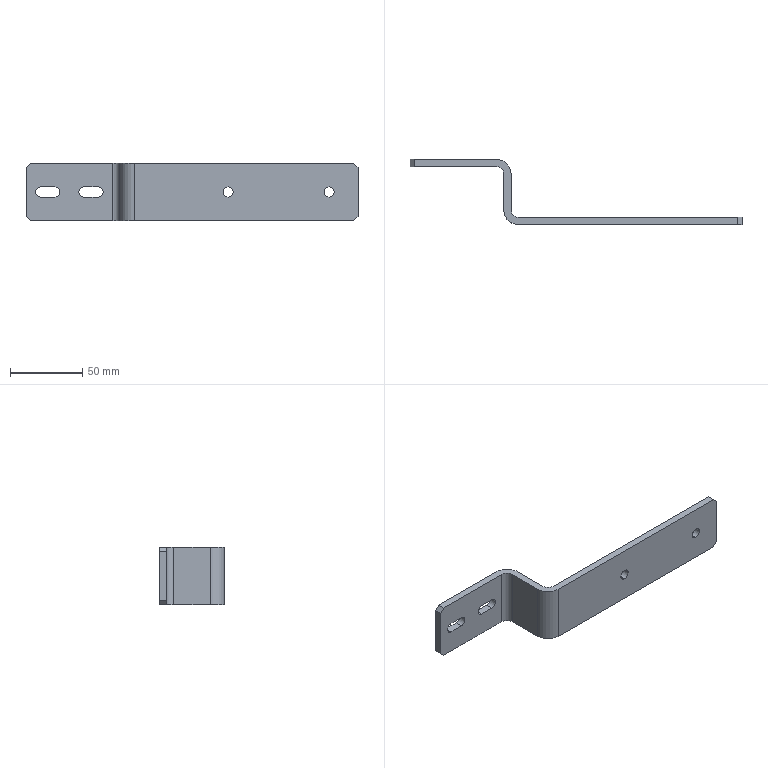Part | SolidWorks | features ICE 2, Chamfer 1, Extrusion 1 | 1 solid | 30 faces | box 230 x 45 x 40 mm | volume 51153 mm3 | plane 18 | cylinder 12 | commonest cylinder face diameters 7 x8 10 x2 20 x2
STEP:
#1=CARTESIAN_POINT('',(140.,-40.,16.5));
#2=VERTEX_POINT('',#1);
#3=CARTESIAN_POINT('',(140.,-40.,23.5));
#4=VERTEX_POINT('',#3);
#5=CARTESIAN_POINT('',(140.,-40.,20.));
#6=DIRECTION('',(0.,1.,0.));
#7=DIRECTION('',(-1.,0.,0.));
#8=AXIS2_PLACEMENT_3D('',#5,#6,#7);
#9=CIRCLE('',#8,3.5);
#10=EDGE_CURVE('',#2,#4,#9,.T.);
#11=ORIENTED_EDGE('',*,*,#10,.F.);
#12=CARTESIAN_POINT('',(140.,-35.,16.5));
#13=VERTEX_POINT('',#12);
#14=CARTESIAN_POINT('',(140.,-75.,16.5));
#15=DIRECTION('',(0.,1.,0.));
#16=VECTOR('',#15,1000.);
#17=LINE('',#14,#16);
#18=EDGE_CURVE('',#2,#13,#17,.T.);
#19=ORIENTED_EDGE('',*,*,#18,.T.);
#20=CARTESIAN_POINT('',(140.,-35.,23.5));
#21=VERTEX_POINT('',#20);
#22=CARTESIAN_POINT('',(140.,-35.,20.));
#23=DIRECTION('',(0.,1.,0.));
#24=DIRECTION('',(0.,0.,1.));
#25=AXIS2_PLACEMENT_3D('',#22,#23,#24);
#26=CIRCLE('',#25,3.5);
#27=EDGE_CURVE('',#13,#21,#26,.T.);
#28=ORIENTED_EDGE('',*,*,#27,.T.);
#29=CARTESIAN_POINT('',(140.,-75.,23.5));
#30=DIRECTION('',(0.,1.,0.));
#31=VECTOR('',#30,1000.);
#32=LINE('',#29,#31);
#33=EDGE_CURVE('',#4,#21,#32,.T.);
#34=ORIENTED_EDGE('',*,*,#33,.F.);
#35=EDGE_LOOP('',(#11,#19,#28,#34));
#36=FACE_OUTER_BOUND('',#35,.T.);
#37=CARTESIAN_POINT('',(140.,-75.,20.));
#38=DIRECTION('',(0.,1.,0.));
#39=DIRECTION('',(0.,0.,1.));
#40=AXIS2_PLACEMENT_3D('',#37,#38,#39);
#41=CYLINDRICAL_SURFACE('',#40,3.5);
#42=ADVANCED_FACE('',(#36),#41,.F.);
#43=CARTESIAN_POINT('',(210.,-40.,16.5));
#44=VERTEX_POINT('',#43);
#45=CARTESIAN_POINT('',(210.,-40.,23.5));
#46=VERTEX_POINT('',#45);
#47=CARTESIAN_POINT('',(210.,-40.,20.));
#48=DIRECTION('',(0.,1.,0.));
#49=DIRECTION('',(-1.,0.,0.));
#50=AXIS2_PLACEMENT_3D('',#47,#48,#49);
#51=CIRCLE('',#50,3.5);
#52=EDGE_CURVE('',#44,#46,#51,.T.);
#53=ORIENTED_EDGE('',*,*,#52,.F.);
#54=CARTESIAN_POINT('',(210.,-35.,16.5));
#55=VERTEX_POINT('',#54);
#56=CARTESIAN_POINT('',(210.,-75.,16.5));
#57=DIRECTION('',(0.,1.,0.));
#58=VECTOR('',#57,1000.);
#59=LINE('',#56,#58);
#60=EDGE_CURVE('',#44,#55,#59,.T.);
#61=ORIENTED_EDGE('',*,*,#60,.T.);
#62=CARTESIAN_POINT('',(210.,-35.,23.5));
#63=VERTEX_POINT('',#62);
#64=CARTESIAN_POINT('',(210.,-35.,20.));
#65=DIRECTION('',(0.,1.,0.));
#66=DIRECTION('',(0.,0.,1.));
#67=AXIS2_PLACEMENT_3D('',#64,#65,#66);
#68=CIRCLE('',#67,3.5);
#69=EDGE_CURVE('',#55,#63,#68,.T.);
#70=ORIENTED_EDGE('',*,*,#69,.T.);
#71=CARTESIAN_POINT('',(210.,-75.,23.5));
#72=DIRECTION('',(0.,1.,0.));
#73=VECTOR('',#72,1000.);
#74=LINE('',#71,#73);
#75=EDGE_CURVE('',#46,#63,#74,.T.);
#76=ORIENTED_EDGE('',*,*,#75,.F.);
#77=EDGE_LOOP('',(#53,#61,#70,#76));
#78=FACE_OUTER_BOUND('',#77,.T.);
#79=CARTESIAN_POINT('',(210.,-75.,20.));
#80=DIRECTION('',(0.,1.,0.));
#81=DIRECTION('',(0.,0.,1.));
#82=AXIS2_PLACEMENT_3D('',#79,#80,#81);
#83=CYLINDRICAL_SURFACE('',#82,3.5);
#84=ADVANCED_FACE('',(#78),#83,.F.);
#85=CARTESIAN_POINT('',(140.,-35.,20.));
#86=DIRECTION('',(0.,1.,0.));
#87=DIRECTION('',(0.,0.,1.));
#88=AXIS2_PLACEMENT_3D('',#85,#86,#87);
#89=CIRCLE('',#88,3.5);
#90=EDGE_CURVE('',#21,#13,#89,.T.);
#91=ORIENTED_EDGE('',*,*,#90,.F.);
#92=ORIENTED_EDGE('',*,*,#27,.F.);
#93=EDGE_LOOP('',(#91,#92));
#94=FACE_BOUND('',#93,.T.);
#95=CARTESIAN_POINT('',(210.,-35.,20.));
#96=DIRECTION('',(0.,1.,0.));
#97=DIRECTION('',(0.,0.,1.));
#98=AXIS2_PLACEMENT_3D('',#95,#96,#97);
#99=CIRCLE('',#98,3.5);
#100=EDGE_CURVE('',#63,#55,#99,.T.);
#101=ORIENTED_EDGE('',*,*,#100,.F.);
#102=ORIENTED_EDGE('',*,*,#69,.F.);
#103=EDGE_LOOP('',(#101,#102));
#104=FACE_BOUND('',#103,.T.);
#105=CARTESIAN_POINT('',(75.,-35.,40.));
#106=VERTEX_POINT('',#105);
#107=CARTESIAN_POINT('',(227.,-35.,40.));
#108=VERTEX_POINT('',#107);
#109=CARTESIAN_POINT('',(75.,-35.,40.));
#110=DIRECTION('',(1.,0.,0.));
#111=VECTOR('',#110,1000.);
#112=LINE('',#109,#111);
#113=EDGE_CURVE('',#106,#108,#112,.T.);
#114=ORIENTED_EDGE('',*,*,#113,.T.);
#115=CARTESIAN_POINT('',(230.,-35.,37.));
#116=VERTEX_POINT('',#115);
#117=CARTESIAN_POINT('',(151.,-35.,116.));
#118=DIRECTION('',(0.7071,0.,-0.7071));
#119=VECTOR('',#118,1000.);
#120=LINE('',#117,#119);
#121=EDGE_CURVE('',#108,#116,#120,.T.);
#122=ORIENTED_EDGE('',*,*,#121,.T.);
#123=CARTESIAN_POINT('',(230.,-35.,3.));
#124=VERTEX_POINT('',#123);
#125=CARTESIAN_POINT('',(230.,-35.,40.));
#126=DIRECTION('',(0.,0.,-1.));
#127=VECTOR('',#126,1000.);
#128=LINE('',#125,#127);
#129=EDGE_CURVE('',#116,#124,#128,.T.);
#130=ORIENTED_EDGE('',*,*,#129,.T.);
#131=CARTESIAN_POINT('',(227.,-35.,0.));
#132=VERTEX_POINT('',#131);
#133=CARTESIAN_POINT('',(171.,-35.,-56.));
#134=DIRECTION('',(-0.7071,0.,-0.7071));
#135=VECTOR('',#134,1000.);
#136=LINE('',#133,#135);
#137=EDGE_CURVE('',#124,#132,#136,.T.);
#138=ORIENTED_EDGE('',*,*,#137,.T.);
#139=CARTESIAN_POINT('',(75.,-35.,0.));
#140=VERTEX_POINT('',#139);
#141=CARTESIAN_POINT('',(75.,-35.,0.));
#142=DIRECTION('',(1.,0.,0.));
#143=VECTOR('',#142,1000.);
#144=LINE('',#141,#143);
#145=EDGE_CURVE('',#140,#132,#144,.T.);
#146=ORIENTED_EDGE('',*,*,#145,.F.);
#147=CARTESIAN_POINT('',(75.,-35.,40.));
#148=DIRECTION('',(0.,0.,-1.));
#149=VECTOR('',#148,1000.);
#150=LINE('',#147,#149);
#151=EDGE_CURVE('',#106,#140,#150,.T.);
#152=ORIENTED_EDGE('',*,*,#151,.F.);
#153=EDGE_LOOP('',(#114,#122,#130,#138,#146,#152));
#154=FACE_OUTER_BOUND('',#153,.T.);
#155=CARTESIAN_POINT('',(75.,-35.,40.));
#156=DIRECTION('',(0.,1.,0.));
#157=DIRECTION('',(0.,0.,1.));
#158=AXIS2_PLACEMENT_3D('',#155,#156,#157);
#159=PLANE('',#158);
#160=ADVANCED_FACE('',(#94,#104,#154),#159,.T.);
#161=CARTESIAN_POINT('',(70.,-30.,0.));
#162=VERTEX_POINT('',#161);
#163=CARTESIAN_POINT('',(75.,-30.,0.));
#164=DIRECTION('',(0.,0.,1.));
#165=DIRECTION('',(1.,0.,0.));
#166=AXIS2_PLACEMENT_3D('',#163,#164,#165);
#167=CIRCLE('',#166,5.);
#168=EDGE_CURVE('',#162,#140,#167,.T.);
#169=ORIENTED_EDGE('',*,*,#168,.F.);
#170=CARTESIAN_POINT('',(70.,-30.,40.));
#171=VERTEX_POINT('',#170);
#172=CARTESIAN_POINT('',(70.,-30.,40.));
#173=DIRECTION('',(0.,0.,-1.));
#174=VECTOR('',#173,1000.);
#175=LINE('',#172,#174);
#176=EDGE_CURVE('',#171,#162,#175,.T.);
#177=ORIENTED_EDGE('',*,*,#176,.F.);
#178=CARTESIAN_POINT('',(75.,-30.,40.));
#179=DIRECTION('',(0.,0.,1.));
#180=DIRECTION('',(1.,0.,0.));
#181=AXIS2_PLACEMENT_3D('',#178,#179,#180);
#182=CIRCLE('',#181,5.);
#183=EDGE_CURVE('',#171,#106,#182,.T.);
#184=ORIENTED_EDGE('',*,*,#183,.T.);
#185=ORIENTED_EDGE('',*,*,#151,.T.);
#186=EDGE_LOOP('',(#169,#177,#184,#185));
#187=FACE_OUTER_BOUND('',#186,.T.);
#188=CARTESIAN_POINT('',(75.,-30.,40.));
#189=DIRECTION('',(0.,0.,-1.));
#190=DIRECTION('',(-1.,0.,0.));
#191=AXIS2_PLACEMENT_3D('',#188,#189,#190);
#192=CYLINDRICAL_SURFACE('',#191,5.);
#193=ADVANCED_FACE('',(#187),#192,.F.);
#194=CARTESIAN_POINT('',(70.,-5.,0.));
#195=VERTEX_POINT('',#194);
#196=CARTESIAN_POINT('',(70.,-5.,0.));
#197=DIRECTION('',(0.,-1.,0.));
#198=VECTOR('',#197,1000.);
#199=LINE('',#196,#198);
#200=EDGE_CURVE('',#195,#162,#199,.T.);
#201=ORIENTED_EDGE('',*,*,#200,.F.);
#202=CARTESIAN_POINT('',(70.,-5.,40.));
#203=VERTEX_POINT('',#202);
#204=CARTESIAN_POINT('',(70.,-5.,40.));
#205=DIRECTION('',(0.,0.,-1.));
#206=VECTOR('',#205,1000.);
#207=LINE('',#204,#206);
#208=EDGE_CURVE('',#203,#195,#207,.T.);
#209=ORIENTED_EDGE('',*,*,#208,.F.);
#210=CARTESIAN_POINT('',(70.,-5.,40.));
#211=DIRECTION('',(0.,-1.,0.));
#212=VECTOR('',#211,1000.);
#213=LINE('',#210,#212);
#214=EDGE_CURVE('',#203,#171,#213,.T.);
#215=ORIENTED_EDGE('',*,*,#214,.T.);
#216=ORIENTED_EDGE('',*,*,#176,.T.);
#217=EDGE_LOOP('',(#201,#209,#215,#216));
#218=FACE_OUTER_BOUND('',#217,.T.);
#219=CARTESIAN_POINT('',(70.,-5.,40.));
#220=DIRECTION('',(1.,0.,0.));
#221=DIRECTION('',(0.,0.,-1.));
#222=AXIS2_PLACEMENT_3D('',#219,#220,#221);
#223=PLANE('',#222);
#224=ADVANCED_FACE('',(#218),#223,.T.);
#225=CARTESIAN_POINT('',(60.,5.,0.));
#226=VERTEX_POINT('',#225);
#227=CARTESIAN_POINT('',(60.,-5.,0.));
#228=DIRECTION('',(0.,0.,-1.));
#229=DIRECTION('',(-1.,0.,0.));
#230=AXIS2_PLACEMENT_3D('',#227,#228,#229);
#231=CIRCLE('',#230,10.);
#232=EDGE_CURVE('',#226,#195,#231,.T.);
#233=ORIENTED_EDGE('',*,*,#232,.F.);
#234=CARTESIAN_POINT('',(60.,5.,40.));
#235=VERTEX_POINT('',#234);
#236=CARTESIAN_POINT('',(60.,5.,40.));
#237=DIRECTION('',(0.,0.,-1.));
#238=VECTOR('',#237,1000.);
#239=LINE('',#236,#238);
#240=EDGE_CURVE('',#235,#226,#239,.T.);
#241=ORIENTED_EDGE('',*,*,#240,.F.);
#242=CARTESIAN_POINT('',(60.,-5.,40.));
#243=DIRECTION('',(0.,0.,-1.));
#244=DIRECTION('',(-1.,0.,0.));
#245=AXIS2_PLACEMENT_3D('',#242,#243,#244);
#246=CIRCLE('',#245,10.);
#247=EDGE_CURVE('',#235,#203,#246,.T.);
#248=ORIENTED_EDGE('',*,*,#247,.T.);
#249=ORIENTED_EDGE('',*,*,#208,.T.);
#250=EDGE_LOOP('',(#233,#241,#248,#249));
#251=FACE_OUTER_BOUND('',#250,.T.);
#252=CARTESIAN_POINT('',(60.,-5.,40.));
#253=DIRECTION('',(0.,0.,-1.));
#254=DIRECTION('',(-1.,0.,0.));
#255=AXIS2_PLACEMENT_3D('',#252,#253,#254);
#256=CYLINDRICAL_SURFACE('',#255,10.);
#257=ADVANCED_FACE('',(#251),#256,.T.);
#258=CARTESIAN_POINT('',(10.,5.,16.5));
#259=VERTEX_POINT('',#258);
#260=CARTESIAN_POINT('',(10.,5.,23.5));
#261=VERTEX_POINT('',#260);
#262=CARTESIAN_POINT('',(10.,5.,20.));
#263=DIRECTION('',(0.,1.,0.));
#264=DIRECTION('',(0.,0.,1.));
#265=AXIS2_PLACEMENT_3D('',#262,#263,#264);
#266=CIRCLE('',#265,3.5);
#267=EDGE_CURVE('',#259,#261,#266,.T.);
#268=ORIENTED_EDGE('',*,*,#267,.F.);
#269=CARTESIAN_POINT('',(20.,5.,16.5));
#270=VERTEX_POINT('',#269);
#271=CARTESIAN_POINT('',(10.,5.,16.5));
#272=DIRECTION('',(-1.,0.,0.));
#273=VECTOR('',#272,1000.);
#274=LINE('',#271,#273);
#275=EDGE_CURVE('',#270,#259,#274,.T.);
#276=ORIENTED_EDGE('',*,*,#275,.F.);
#277=CARTESIAN_POINT('',(20.,5.,23.5));
#278=VERTEX_POINT('',#277);
#279=CARTESIAN_POINT('',(20.,5.,20.));
#280=DIRECTION('',(0.,1.,0.));
#281=DIRECTION('',(0.,0.,1.));
#282=AXIS2_PLACEMENT_3D('',#279,#280,#281);
#283=CIRCLE('',#282,3.5);
#284=EDGE_CURVE('',#278,#270,#283,.T.);
#285=ORIENTED_EDGE('',*,*,#284,.F.);
#286=CARTESIAN_POINT('',(10.,5.,23.5));
#287=DIRECTION('',(1.,0.,0.));
#288=VECTOR('',#287,1000.);
#289=LINE('',#286,#288);
#290=EDGE_CURVE('',#261,#278,#289,.T.);
#291=ORIENTED_EDGE('',*,*,#290,.F.);
#292=EDGE_LOOP('',(#268,#276,#285,#291));
#293=FACE_BOUND('',#292,.T.);
#294=CARTESIAN_POINT('',(40.,5.,16.5));
#295=VERTEX_POINT('',#294);
#296=CARTESIAN_POINT('',(40.,5.,23.5));
#297=VERTEX_POINT('',#296);
#298=CARTESIAN_POINT('',(40.,5.,20.));
#299=DIRECTION('',(0.,1.,0.));
#300=DIRECTION('',(0.,0.,1.));
#301=AXIS2_PLACEMENT_3D('',#298,#299,#300);
#302=CIRCLE('',#301,3.5);
#303=EDGE_CURVE('',#295,#297,#302,.T.);
#304=ORIENTED_EDGE('',*,*,#303,.F.);
#305=CARTESIAN_POINT('',(50.,5.,16.5));
#306=VERTEX_POINT('',#305);
#307=CARTESIAN_POINT('',(40.,5.,16.5));
#308=DIRECTION('',(-1.,0.,0.));
#309=VECTOR('',#308,1000.);
#310=LINE('',#307,#309);
#311=EDGE_CURVE('',#306,#295,#310,.T.);
#312=ORIENTED_EDGE('',*,*,#311,.F.);
#313=CARTESIAN_POINT('',(50.,5.,23.5));
#314=VERTEX_POINT('',#313);
#315=CARTESIAN_POINT('',(50.,5.,20.));
#316=DIRECTION('',(0.,1.,0.));
#317=DIRECTION('',(0.,0.,1.));
#318=AXIS2_PLACEMENT_3D('',#315,#316,#317);
#319=CIRCLE('',#318,3.5);
#320=EDGE_CURVE('',#314,#306,#319,.T.);
#321=ORIENTED_EDGE('',*,*,#320,.F.);
#322=CARTESIAN_POINT('',(40.,5.,23.5));
#323=DIRECTION('',(1.,0.,0.));
#324=VECTOR('',#323,1000.);
#325=LINE('',#322,#324);
#326=EDGE_CURVE('',#297,#314,#325,.T.);
#327=ORIENTED_EDGE('',*,*,#326,.F.);
#328=EDGE_LOOP('',(#304,#312,#321,#327));
#329=FACE_BOUND('',#328,.T.);
#330=CARTESIAN_POINT('',(0.,5.,37.));
#331=VERTEX_POINT('',#330);
#332=CARTESIAN_POINT('',(0.,5.,3.));
#333=VERTEX_POINT('',#332);
#334=CARTESIAN_POINT('',(0.,5.,40.));
#335=DIRECTION('',(0.,0.,-1.));
#336=VECTOR('',#335,1000.);
#337=LINE('',#334,#336);
#338=EDGE_CURVE('',#331,#333,#337,.T.);
#339=ORIENTED_EDGE('',*,*,#338,.F.);
#340=CARTESIAN_POINT('',(3.,5.,40.));
#341=VERTEX_POINT('',#340);
#342=CARTESIAN_POINT('',(1.5,5.,38.5));
#343=DIRECTION('',(0.7071,0.,0.7071));
#344=VECTOR('',#343,1000.);
#345=LINE('',#342,#344);
#346=EDGE_CURVE('',#331,#341,#345,.T.);
#347=ORIENTED_EDGE('',*,*,#346,.T.);
#348=CARTESIAN_POINT('',(0.,5.,40.));
#349=DIRECTION('',(1.,0.,0.));
#350=VECTOR('',#349,1000.);
#351=LINE('',#348,#350);
#352=EDGE_CURVE('',#341,#235,#351,.T.);
#353=ORIENTED_EDGE('',*,*,#352,.T.);
#354=ORIENTED_EDGE('',*,*,#240,.T.);
#355=CARTESIAN_POINT('',(3.,5.,0.));
#356=VERTEX_POINT('',#355);
#357=CARTESIAN_POINT('',(0.,5.,0.));
#358=DIRECTION('',(1.,0.,0.));
#359=VECTOR('',#358,1000.);
#360=LINE('',#357,#359);
#361=EDGE_CURVE('',#356,#226,#360,.T.);
#362=ORIENTED_EDGE('',*,*,#361,.F.);
#363=CARTESIAN_POINT('',(-18.5,5.,21.5));
#364=DIRECTION('',(-0.7071,0.,0.7071));
#365=VECTOR('',#364,1000.);
#366=LINE('',#363,#365);
#367=EDGE_CURVE('',#356,#333,#366,.T.);
#368=ORIENTED_EDGE('',*,*,#367,.T.);
#369=EDGE_LOOP('',(#339,#347,#353,#354,#362,#368));
#370=FACE_OUTER_BOUND('',#369,.T.);
#371=CARTESIAN_POINT('',(0.,5.,40.));
#372=DIRECTION('',(0.,1.,0.));
#373=DIRECTION('',(0.,0.,1.));
#374=AXIS2_PLACEMENT_3D('',#371,#372,#373);
#375=PLANE('',#374);
#376=ADVANCED_FACE('',(#293,#329,#370),#375,.T.);
#377=CARTESIAN_POINT('',(0.,0.,37.));
#378=VERTEX_POINT('',#377);
#379=CARTESIAN_POINT('',(0.,0.,3.));
#380=VERTEX_POINT('',#379);
#381=CARTESIAN_POINT('',(0.,0.,40.));
#382=DIRECTION('',(0.,0.,-1.));
#383=VECTOR('',#382,1000.);
#384=LINE('',#381,#383);
#385=EDGE_CURVE('',#378,#380,#384,.T.);
#386=ORIENTED_EDGE('',*,*,#385,.F.);
#387=CARTESIAN_POINT('',(0.,5.,37.));
#388=DIRECTION('',(0.,1.,0.));
#389=VECTOR('',#388,1000.);
#390=LINE('',#387,#389);
#391=EDGE_CURVE('',#378,#331,#390,.T.);
#392=ORIENTED_EDGE('',*,*,#391,.T.);
#393=ORIENTED_EDGE('',*,*,#338,.T.);
#394=CARTESIAN_POINT('',(0.,5.,3.));
#395=DIRECTION('',(0.,-1.,0.));
#396=VECTOR('',#395,1000.);
#397=LINE('',#394,#396);
#398=EDGE_CURVE('',#333,#380,#397,.T.);
#399=ORIENTED_EDGE('',*,*,#398,.T.);
#400=EDGE_LOOP('',(#386,#392,#393,#399));
#401=FACE_OUTER_BOUND('',#400,.T.);
#402=CARTESIAN_POINT('',(0.,5.,40.));
#403=DIRECTION('',(1.,0.,0.));
#404=DIRECTION('',(0.,0.,-1.));
#405=AXIS2_PLACEMENT_3D('',#402,#403,#404);
#406=PLANE('',#405);
#407=ADVANCED_FACE('',(#401),#406,.F.);
#408=CARTESIAN_POINT('',(20.,0.,16.5));
#409=VERTEX_POINT('',#408);
#410=CARTESIAN_POINT('',(10.,0.,16.5));
#411=VERTEX_POINT('',#410);
#412=CARTESIAN_POINT('',(0.,0.,16.5));
#413=DIRECTION('',(-1.,0.,0.));
#414=VECTOR('',#413,1000.);
#415=LINE('',#412,#414);
#416=EDGE_CURVE('',#409,#411,#415,.T.);
#417=ORIENTED_EDGE('',*,*,#416,.T.);
#418=CARTESIAN_POINT('',(10.,0.,23.5));
#419=VERTEX_POINT('',#418);
#420=CARTESIAN_POINT('',(10.,0.,20.));
#421=DIRECTION('',(0.,1.,0.));
#422=DIRECTION('',(0.,0.,1.));
#423=AXIS2_PLACEMENT_3D('',#420,#421,#422);
#424=CIRCLE('',#423,3.5);
#425=EDGE_CURVE('',#411,#419,#424,.T.);
#426=ORIENTED_EDGE('',*,*,#425,.T.);
#427=CARTESIAN_POINT('',(20.,0.,23.5));
#428=VERTEX_POINT('',#427);
#429=CARTESIAN_POINT('',(0.,0.,23.5));
#430=DIRECTION('',(1.,0.,0.));
#431=VECTOR('',#430,1000.);
#432=LINE('',#429,#431);
#433=EDGE_CURVE('',#419,#428,#432,.T.);
#434=ORIENTED_EDGE('',*,*,#433,.T.);
#435=CARTESIAN_POINT('',(20.,0.,20.));
#436=DIRECTION('',(0.,1.,0.));
#437=DIRECTION('',(0.,0.,1.));
#438=AXIS2_PLACEMENT_3D('',#435,#436,#437);
#439=CIRCLE('',#438,3.5);
#440=EDGE_CURVE('',#428,#409,#439,.T.);
#441=ORIENTED_EDGE('',*,*,#440,.T.);
#442=EDGE_LOOP('',(#417,#426,#434,#441));
#443=FACE_BOUND('',#442,.T.);
#444=CARTESIAN_POINT('',(50.,0.,16.5));
#445=VERTEX_POINT('',#444);
#446=CARTESIAN_POINT('',(40.,0.,16.5));
#447=VERTEX_POINT('',#446);
#448=CARTESIAN_POINT('',(0.,0.,16.5));
#449=DIRECTION('',(-1.,0.,0.));
#450=VECTOR('',#449,1000.);
#451=LINE('',#448,#450);
#452=EDGE_CURVE('',#445,#447,#451,.T.);
#453=ORIENTED_EDGE('',*,*,#452,.T.);
#454=CARTESIAN_POINT('',(40.,0.,23.5));
#455=VERTEX_POINT('',#454);
#456=CARTESIAN_POINT('',(40.,0.,20.));
#457=DIRECTION('',(0.,1.,0.));
#458=DIRECTION('',(0.,0.,1.));
#459=AXIS2_PLACEMENT_3D('',#456,#457,#458);
#460=CIRCLE('',#459,3.5);
#461=EDGE_CURVE('',#447,#455,#460,.T.);
#462=ORIENTED_EDGE('',*,*,#461,.T.);
#463=CARTESIAN_POINT('',(50.,0.,23.5));
#464=VERTEX_POINT('',#463);
#465=CARTESIAN_POINT('',(0.,0.,23.5));
#466=DIRECTION('',(1.,0.,0.));
#467=VECTOR('',#466,1000.);
#468=LINE('',#465,#467);
#469=EDGE_CURVE('',#455,#464,#468,.T.);
#470=ORIENTED_EDGE('',*,*,#469,.T.);
#471=CARTESIAN_POINT('',(50.,0.,20.));
#472=DIRECTION('',(0.,1.,0.));
#473=DIRECTION('',(0.,0.,1.));
#474=AXIS2_PLACEMENT_3D('',#471,#472,#473);
#475=CIRCLE('',#474,3.5);
#476=EDGE_CURVE('',#464,#445,#475,.T.);
#477=ORIENTED_EDGE('',*,*,#476,.T.);
#478=EDGE_LOOP('',(#453,#462,#470,#477));
#479=FACE_BOUND('',#478,.T.);
#480=CARTESIAN_POINT('',(3.,0.,40.));
#481=VERTEX_POINT('',#480);
#482=CARTESIAN_POINT('',(60.,0.,40.));
#483=VERTEX_POINT('',#482);
#484=CARTESIAN_POINT('',(0.,0.,40.));
#485=DIRECTION('',(1.,0.,0.));
#486=VECTOR('',#485,1000.);
#487=LINE('',#484,#486);
#488=EDGE_CURVE('',#481,#483,#487,.T.);
#489=ORIENTED_EDGE('',*,*,#488,.F.);
#490=CARTESIAN_POINT('',(3.,0.,40.));
#491=DIRECTION('',(-0.7071,0.,-0.7071));
#492=VECTOR('',#491,1000.);
#493=LINE('',#490,#492);
#494=EDGE_CURVE('',#481,#378,#493,.T.);
#495=ORIENTED_EDGE('',*,*,#494,.T.);
#496=ORIENTED_EDGE('',*,*,#385,.T.);
#497=CARTESIAN_POINT('',(3.,0.,0.));
#498=VERTEX_POINT('',#497);
#499=CARTESIAN_POINT('',(0.,0.,3.));
#500=DIRECTION('',(0.7071,0.,-0.7071));
#501=VECTOR('',#500,1000.);
#502=LINE('',#499,#501);
#503=EDGE_CURVE('',#380,#498,#502,.T.);
#504=ORIENTED_EDGE('',*,*,#503,.T.);
#505=CARTESIAN_POINT('',(60.,0.,0.));
#506=VERTEX_POINT('',#505);
#507=CARTESIAN_POINT('',(0.,0.,0.));
#508=DIRECTION('',(1.,0.,0.));
#509=VECTOR('',#508,1000.);
#510=LINE('',#507,#509);
#511=EDGE_CURVE('',#498,#506,#510,.T.);
#512=ORIENTED_EDGE('',*,*,#511,.T.);
#513=CARTESIAN_POINT('',(60.,0.,40.));
#514=DIRECTION('',(0.,0.,-1.));
#515=VECTOR('',#514,1000.);
#516=LINE('',#513,#515);
#517=EDGE_CURVE('',#483,#506,#516,.T.);
#518=ORIENTED_EDGE('',*,*,#517,.F.);
#519=EDGE_LOOP('',(#489,#495,#496,#504,#512,#518));
#520=FACE_OUTER_BOUND('',#519,.T.);
#521=CARTESIAN_POINT('',(0.,0.,40.));
#522=DIRECTION('',(0.,1.,0.));
#523=DIRECTION('',(0.,0.,1.));
#524=AXIS2_PLACEMENT_3D('',#521,#522,#523);
#525=PLANE('',#524);
#526=ADVANCED_FACE('',(#443,#479,#520),#525,.F.);
#527=CARTESIAN_POINT('',(65.,-5.,0.));
#528=VERTEX_POINT('',#527);
#529=CARTESIAN_POINT('',(60.,-5.,0.));
#530=DIRECTION('',(0.,0.,-1.));
#531=DIRECTION('',(-1.,0.,0.));
#532=AXIS2_PLACEMENT_3D('',#529,#530,#531);
#533=CIRCLE('',#532,5.);
#534=EDGE_CURVE('',#506,#528,#533,.T.);
#535=ORIENTED_EDGE('',*,*,#534,.T.);
#536=CARTESIAN_POINT('',(65.,-5.,40.));
#537=VERTEX_POINT('',#536);
#538=CARTESIAN_POINT('',(65.,-5.,40.));
#539=DIRECTION('',(0.,0.,-1.));
#540=VECTOR('',#539,1000.);
#541=LINE('',#538,#540);
#542=EDGE_CURVE('',#537,#528,#541,.T.);
#543=ORIENTED_EDGE('',*,*,#542,.F.);
#544=CARTESIAN_POINT('',(60.,-5.,40.));
#545=DIRECTION('',(0.,0.,-1.));
#546=DIRECTION('',(-1.,0.,0.));
#547=AXIS2_PLACEMENT_3D('',#544,#545,#546);
#548=CIRCLE('',#547,5.);
#549=EDGE_CURVE('',#483,#537,#548,.T.);
#550=ORIENTED_EDGE('',*,*,#549,.F.);
#551=ORIENTED_EDGE('',*,*,#517,.T.);
#552=EDGE_LOOP('',(#535,#543,#550,#551));
#553=FACE_OUTER_BOUND('',#552,.T.);
#554=CARTESIAN_POINT('',(60.,-5.,40.));
#555=DIRECTION('',(0.,0.,-1.));
#556=DIRECTION('',(-1.,0.,0.));
#557=AXIS2_PLACEMENT_3D('',#554,#555,#556);
#558=CYLINDRICAL_SURFACE('',#557,5.);
#559=ADVANCED_FACE('',(#553),#558,.F.);
#560=CARTESIAN_POINT('',(65.,-30.,0.));
#561=VERTEX_POINT('',#560);
#562=CARTESIAN_POINT('',(65.,-5.,0.));
#563=DIRECTION('',(0.,-1.,0.));
#564=VECTOR('',#563,1000.);
#565=LINE('',#562,#564);
#566=EDGE_CURVE('',#528,#561,#565,.T.);
#567=ORIENTED_EDGE('',*,*,#566,.T.);
#568=CARTESIAN_POINT('',(65.,-30.,40.));
#569=VERTEX_POINT('',#568);
#570=CARTESIAN_POINT('',(65.,-30.,40.));
#571=DIRECTION('',(0.,0.,-1.));
#572=VECTOR('',#571,1000.);
#573=LINE('',#570,#572);
#574=EDGE_CURVE('',#569,#561,#573,.T.);
#575=ORIENTED_EDGE('',*,*,#574,.F.);
#576=CARTESIAN_POINT('',(65.,-5.,40.));
#577=DIRECTION('',(0.,-1.,0.));
#578=VECTOR('',#577,1000.);
#579=LINE('',#576,#578);
#580=EDGE_CURVE('',#537,#569,#579,.T.);
#581=ORIENTED_EDGE('',*,*,#580,.F.);
#582=ORIENTED_EDGE('',*,*,#542,.T.);
#583=EDGE_LOOP('',(#567,#575,#581,#582));
#584=FACE_OUTER_BOUND('',#583,.T.);
#585=CARTESIAN_POINT('',(65.,-5.,40.));
#586=DIRECTION('',(1.,0.,0.));
#587=DIRECTION('',(0.,1.,0.));
#588=AXIS2_PLACEMENT_3D('',#585,#586,#587);
#589=PLANE('',#588);
#590=ADVANCED_FACE('',(#584),#589,.F.);
#591=CARTESIAN_POINT('',(75.,-40.,0.));
#592=VERTEX_POINT('',#591);
#593=CARTESIAN_POINT('',(75.,-30.,0.));
#594=DIRECTION('',(0.,0.,1.));
#595=DIRECTION('',(1.,0.,0.));
#596=AXIS2_PLACEMENT_3D('',#593,#594,#595);
#597=CIRCLE('',#596,10.);
#598=EDGE_CURVE('',#561,#592,#597,.T.);
#599=ORIENTED_EDGE('',*,*,#598,.T.);
#600=CARTESIAN_POINT('',(75.,-40.,40.));
#601=VERTEX_POINT('',#600);
#602=CARTESIAN_POINT('',(75.,-40.,40.));
#603=DIRECTION('',(0.,0.,-1.));
#604=VECTOR('',#603,1000.);
#605=LINE('',#602,#604);
#606=EDGE_CURVE('',#601,#592,#605,.T.);
#607=ORIENTED_EDGE('',*,*,#606,.F.);
#608=CARTESIAN_POINT('',(75.,-30.,40.));
#609=DIRECTION('',(0.,0.,1.));
#610=DIRECTION('',(1.,0.,0.));
#611=AXIS2_PLACEMENT_3D('',#608,#609,#610);
#612=CIRCLE('',#611,10.);
#613=EDGE_CURVE('',#569,#601,#612,.T.);
#614=ORIENTED_EDGE('',*,*,#613,.F.);
#615=ORIENTED_EDGE('',*,*,#574,.T.);
#616=EDGE_LOOP('',(#599,#607,#614,#615));
#617=FACE_OUTER_BOUND('',#616,.T.);
#618=CARTESIAN_POINT('',(75.,-30.,40.));
#619=DIRECTION('',(0.,0.,-1.));
#620=DIRECTION('',(-1.,0.,0.));
#621=AXIS2_PLACEMENT_3D('',#618,#619,#620);
#622=CYLINDRICAL_SURFACE('',#621,10.);
#623=ADVANCED_FACE('',(#617),#622,.T.);
#624=CARTESIAN_POINT('',(140.,-40.,20.));
#625=DIRECTION('',(0.,1.,0.));
#626=DIRECTION('',(-1.,0.,0.));
#627=AXIS2_PLACEMENT_3D('',#624,#625,#626);
#628=CIRCLE('',#627,3.5);
#629=EDGE_CURVE('',#4,#2,#628,.T.);
#630=ORIENTED_EDGE('',*,*,#629,.T.);
#631=ORIENTED_EDGE('',*,*,#10,.T.);
#632=EDGE_LOOP('',(#630,#631));
#633=FACE_BOUND('',#632,.T.);
#634=CARTESIAN_POINT('',(210.,-40.,20.));
#635=DIRECTION('',(0.,1.,0.));
#636=DIRECTION('',(-1.,0.,0.));
#637=AXIS2_PLACEMENT_3D('',#634,#635,#636);
#638=CIRCLE('',#637,3.5);
#639=EDGE_CURVE('',#46,#44,#638,.T.);
#640=ORIENTED_EDGE('',*,*,#639,.T.);
#641=ORIENTED_EDGE('',*,*,#52,.T.);
#642=EDGE_LOOP('',(#640,#641));
#643=FACE_BOUND('',#642,.T.);
#644=CARTESIAN_POINT('',(230.,-40.,37.));
#645=VERTEX_POINT('',#644);
#646=CARTESIAN_POINT('',(230.,-40.,3.));
#647=VERTEX_POINT('',#646);
#648=CARTESIAN_POINT('',(230.,-40.,40.));
#649=DIRECTION('',(0.,0.,-1.));
#650=VECTOR('',#649,1000.);
#651=LINE('',#648,#650);
#652=EDGE_CURVE('',#645,#647,#651,.T.);
#653=ORIENTED_EDGE('',*,*,#652,.F.);
#654=CARTESIAN_POINT('',(227.,-40.,40.));
#655=VERTEX_POINT('',#654);
#656=CARTESIAN_POINT('',(230.,-40.,37.));
#657=DIRECTION('',(-0.7071,0.,0.7071));
#658=VECTOR('',#657,1000.);
#659=LINE('',#656,#658);
#660=EDGE_CURVE('',#645,#655,#659,.T.);
#661=ORIENTED_EDGE('',*,*,#660,.T.);
#662=CARTESIAN_POINT('',(75.,-40.,40.));
#663=DIRECTION('',(1.,0.,0.));
#664=VECTOR('',#663,1000.);
#665=LINE('',#662,#664);
#666=EDGE_CURVE('',#601,#655,#665,.T.);
#667=ORIENTED_EDGE('',*,*,#666,.F.);
#668=ORIENTED_EDGE('',*,*,#606,.T.);
#669=CARTESIAN_POINT('',(227.,-40.,0.));
#670=VERTEX_POINT('',#669);
#671=CARTESIAN_POINT('',(75.,-40.,0.));
#672=DIRECTION('',(1.,0.,0.));
#673=VECTOR('',#672,1000.);
#674=LINE('',#671,#673);
#675=EDGE_CURVE('',#592,#670,#674,.T.);
#676=ORIENTED_EDGE('',*,*,#675,.T.);
#677=CARTESIAN_POINT('',(227.,-40.,0.));
#678=DIRECTION('',(0.7071,0.,0.7071));
#679=VECTOR('',#678,1000.);
#680=LINE('',#677,#679);
#681=EDGE_CURVE('',#670,#647,#680,.T.);
#682=ORIENTED_EDGE('',*,*,#681,.T.);
#683=EDGE_LOOP('',(#653,#661,#667,#668,#676,#682));
#684=FACE_OUTER_BOUND('',#683,.T.);
#685=CARTESIAN_POINT('',(75.,-40.,40.));
#686=DIRECTION('',(0.,1.,0.));
#687=DIRECTION('',(-1.,0.,0.));
#688=AXIS2_PLACEMENT_3D('',#685,#686,#687);
#689=PLANE('',#688);
#690=ADVANCED_FACE('',(#633,#643,#684),#689,.F.);
#691=ORIENTED_EDGE('',*,*,#129,.F.);
#692=CARTESIAN_POINT('',(230.,-35.,37.));
#693=DIRECTION('',(0.,-1.,0.));
#694=VECTOR('',#693,1000.);
#695=LINE('',#692,#694);
#696=EDGE_CURVE('',#116,#645,#695,.T.);
#697=ORIENTED_EDGE('',*,*,#696,.T.);
#698=ORIENTED_EDGE('',*,*,#652,.T.);
#699=CARTESIAN_POINT('',(230.,-35.,3.));
#700=DIRECTION('',(0.,1.,0.));
#701=VECTOR('',#700,1000.);
#702=LINE('',#699,#701);
#703=EDGE_CURVE('',#647,#124,#702,.T.);
#704=ORIENTED_EDGE('',*,*,#703,.T.);
#705=EDGE_LOOP('',(#691,#697,#698,#704));
#706=FACE_OUTER_BOUND('',#705,.T.);
#707=CARTESIAN_POINT('',(230.,-35.,40.));
#708=DIRECTION('',(1.,0.,0.));
#709=DIRECTION('',(0.,0.,-1.));
#710=AXIS2_PLACEMENT_3D('',#707,#708,#709);
#711=PLANE('',#710);
#712=ADVANCED_FACE('',(#706),#711,.T.);
#713=ORIENTED_EDGE('',*,*,#352,.F.);
#714=CARTESIAN_POINT('',(3.,0.,40.));
#715=DIRECTION('',(0.,-1.,0.));
#716=VECTOR('',#715,1000.);
#717=LINE('',#714,#716);
#718=EDGE_CURVE('',#341,#481,#717,.T.);
#719=ORIENTED_EDGE('',*,*,#718,.T.);
#720=ORIENTED_EDGE('',*,*,#488,.T.);
#721=ORIENTED_EDGE('',*,*,#549,.T.);
#722=ORIENTED_EDGE('',*,*,#580,.T.);
#723=ORIENTED_EDGE('',*,*,#613,.T.);
#724=ORIENTED_EDGE('',*,*,#666,.T.);
#725=CARTESIAN_POINT('',(227.,-30.,40.));
#726=DIRECTION('',(0.,1.,0.));
#727=VECTOR('',#726,1000.);
#728=LINE('',#725,#727);
#729=EDGE_CURVE('',#655,#108,#728,.T.);
#730=ORIENTED_EDGE('',*,*,#729,.T.);
#731=ORIENTED_EDGE('',*,*,#113,.F.);
#732=ORIENTED_EDGE('',*,*,#183,.F.);
#733=ORIENTED_EDGE('',*,*,#214,.F.);
#734=ORIENTED_EDGE('',*,*,#247,.F.);
#735=EDGE_LOOP('',(#713,#719,#720,#721,#722,#723,#724,#730,#731,#732,#733,#734));
#736=FACE_OUTER_BOUND('',#735,.T.);
#737=CARTESIAN_POINT('',(75.,-30.,40.));
#738=DIRECTION('',(0.,0.,1.));
#739=DIRECTION('',(1.,0.,0.));
#740=AXIS2_PLACEMENT_3D('',#737,#738,#739);
#741=PLANE('',#740);
#742=ADVANCED_FACE('',(#736),#741,.T.);
#743=ORIENTED_EDGE('',*,*,#511,.F.);
#744=CARTESIAN_POINT('',(3.,-30.,0.));
#745=DIRECTION('',(0.,1.,0.));
#746=VECTOR('',#745,1000.);
#747=LINE('',#744,#746);
#748=EDGE_CURVE('',#498,#356,#747,.T.);
#749=ORIENTED_EDGE('',*,*,#748,.T.);
#750=ORIENTED_EDGE('',*,*,#361,.T.);
#751=ORIENTED_EDGE('',*,*,#232,.T.);
#752=ORIENTED_EDGE('',*,*,#200,.T.);
#753=ORIENTED_EDGE('',*,*,#168,.T.);
#754=ORIENTED_EDGE('',*,*,#145,.T.);
#755=CARTESIAN_POINT('',(227.,-40.,0.));
#756=DIRECTION('',(0.,-1.,0.));
#757=VECTOR('',#756,1000.);
#758=LINE('',#755,#757);
#759=EDGE_CURVE('',#132,#670,#758,.T.);
#760=ORIENTED_EDGE('',*,*,#759,.T.);
#761=ORIENTED_EDGE('',*,*,#675,.F.);
#762=ORIENTED_EDGE('',*,*,#598,.F.);
#763=ORIENTED_EDGE('',*,*,#566,.F.);
#764=ORIENTED_EDGE('',*,*,#534,.F.);
#765=EDGE_LOOP('',(#743,#749,#750,#751,#752,#753,#754,#760,#761,#762,#763,#764));
#766=FACE_OUTER_BOUND('',#765,.T.);
#767=CARTESIAN_POINT('',(75.,-30.,0.));
#768=DIRECTION('',(0.,0.,1.));
#769=DIRECTION('',(1.,0.,0.));
#770=AXIS2_PLACEMENT_3D('',#767,#768,#769);
#771=PLANE('',#770);
#772=ADVANCED_FACE('',(#766),#771,.F.);
#773=CARTESIAN_POINT('',(40.,-35.,16.5));
#774=DIRECTION('',(0.,1.,0.));
#775=VECTOR('',#774,1000.);
#776=LINE('',#773,#775);
#777=EDGE_CURVE('',#447,#295,#776,.T.);
#778=ORIENTED_EDGE('',*,*,#777,.T.);
#779=ORIENTED_EDGE('',*,*,#303,.T.);
#780=CARTESIAN_POINT('',(40.,-35.,23.5));
#781=DIRECTION('',(0.,1.,0.));
#782=VECTOR('',#781,1000.);
#783=LINE('',#780,#782);
#784=EDGE_CURVE('',#455,#297,#783,.T.);
#785=ORIENTED_EDGE('',*,*,#784,.F.);
#786=ORIENTED_EDGE('',*,*,#461,.F.);
#787=EDGE_LOOP('',(#778,#779,#785,#786));
#788=FACE_OUTER_BOUND('',#787,.T.);
#789=CARTESIAN_POINT('',(40.,-35.,20.));
#790=DIRECTION('',(0.,1.,0.));
#791=DIRECTION('',(0.,0.,1.));
#792=AXIS2_PLACEMENT_3D('',#789,#790,#791);
#793=CYLINDRICAL_SURFACE('',#792,3.5);
#794=ADVANCED_FACE('',(#788),#793,.F.);
#795=CARTESIAN_POINT('',(50.,-35.,16.5));
#796=DIRECTION('',(0.,1.,0.));
#797=VECTOR('',#796,1000.);
#798=LINE('',#795,#797);
#799=EDGE_CURVE('',#445,#306,#798,.T.);
#800=ORIENTED_EDGE('',*,*,#799,.T.);
#801=ORIENTED_EDGE('',*,*,#311,.T.);
#802=ORIENTED_EDGE('',*,*,#777,.F.);
#803=ORIENTED_EDGE('',*,*,#452,.F.);
#804=EDGE_LOOP('',(#800,#801,#802,#803));
#805=FACE_OUTER_BOUND('',#804,.T.);
#806=CARTESIAN_POINT('',(40.,-35.,16.5));
#807=DIRECTION('',(0.,0.,-1.));
#808=DIRECTION('',(-1.,0.,0.));
#809=AXIS2_PLACEMENT_3D('',#806,#807,#808);
#810=PLANE('',#809);
#811=ADVANCED_FACE('',(#805),#810,.F.);
#812=CARTESIAN_POINT('',(50.,-35.,23.5));
#813=DIRECTION('',(0.,1.,0.));
#814=VECTOR('',#813,1000.);
#815=LINE('',#812,#814);
#816=EDGE_CURVE('',#464,#314,#815,.T.);
#817=ORIENTED_EDGE('',*,*,#816,.T.);
#818=ORIENTED_EDGE('',*,*,#320,.T.);
#819=ORIENTED_EDGE('',*,*,#799,.F.);
#820=ORIENTED_EDGE('',*,*,#476,.F.);
#821=EDGE_LOOP('',(#817,#818,#819,#820));
#822=FACE_OUTER_BOUND('',#821,.T.);
#823=CARTESIAN_POINT('',(50.,-35.,20.));
#824=DIRECTION('',(0.,1.,0.));
#825=DIRECTION('',(0.,0.,1.));
#826=AXIS2_PLACEMENT_3D('',#823,#824,#825);
#827=CYLINDRICAL_SURFACE('',#826,3.5);
#828=ADVANCED_FACE('',(#822),#827,.F.);
#829=ORIENTED_EDGE('',*,*,#784,.T.);
#830=ORIENTED_EDGE('',*,*,#326,.T.);
#831=ORIENTED_EDGE('',*,*,#816,.F.);
#832=ORIENTED_EDGE('',*,*,#469,.F.);
#833=EDGE_LOOP('',(#829,#830,#831,#832));
#834=FACE_OUTER_BOUND('',#833,.T.);
#835=CARTESIAN_POINT('',(40.,-35.,23.5));
#836=DIRECTION('',(0.,0.,1.));
#837=DIRECTION('',(1.,0.,0.));
#838=AXIS2_PLACEMENT_3D('',#835,#836,#837);
#839=PLANE('',#838);
#840=ADVANCED_FACE('',(#834),#839,.F.);
#841=CARTESIAN_POINT('',(10.,-35.,16.5));
#842=DIRECTION('',(0.,1.,0.));
#843=VECTOR('',#842,1000.);
#844=LINE('',#841,#843);
#845=EDGE_CURVE('',#411,#259,#844,.T.);
#846=ORIENTED_EDGE('',*,*,#845,.T.);
#847=ORIENTED_EDGE('',*,*,#267,.T.);
#848=CARTESIAN_POINT('',(10.,-35.,23.5));
#849=DIRECTION('',(0.,1.,0.));
#850=VECTOR('',#849,1000.);
#851=LINE('',#848,#850);
#852=EDGE_CURVE('',#419,#261,#851,.T.);
#853=ORIENTED_EDGE('',*,*,#852,.F.);
#854=ORIENTED_EDGE('',*,*,#425,.F.);
#855=EDGE_LOOP('',(#846,#847,#853,#854));
#856=FACE_OUTER_BOUND('',#855,.T.);
#857=CARTESIAN_POINT('',(10.,-35.,20.));
#858=DIRECTION('',(0.,1.,0.));
#859=DIRECTION('',(0.,0.,1.));
#860=AXIS2_PLACEMENT_3D('',#857,#858,#859);
#861=CYLINDRICAL_SURFACE('',#860,3.5);
#862=ADVANCED_FACE('',(#856),#861,.F.);
#863=CARTESIAN_POINT('',(20.,-35.,16.5));
#864=DIRECTION('',(0.,1.,0.));
#865=VECTOR('',#864,1000.);
#866=LINE('',#863,#865);
#867=EDGE_CURVE('',#409,#270,#866,.T.);
#868=ORIENTED_EDGE('',*,*,#867,.T.);
#869=ORIENTED_EDGE('',*,*,#275,.T.);
#870=ORIENTED_EDGE('',*,*,#845,.F.);
#871=ORIENTED_EDGE('',*,*,#416,.F.);
#872=EDGE_LOOP('',(#868,#869,#870,#871));
#873=FACE_OUTER_BOUND('',#872,.T.);
#874=CARTESIAN_POINT('',(10.,-35.,16.5));
#875=DIRECTION('',(0.,0.,-1.));
#876=DIRECTION('',(-1.,0.,0.));
#877=AXIS2_PLACEMENT_3D('',#874,#875,#876);
#878=PLANE('',#877);
#879=ADVANCED_FACE('',(#873),#878,.F.);
#880=CARTESIAN_POINT('',(20.,-35.,23.5));
#881=DIRECTION('',(0.,1.,0.));
#882=VECTOR('',#881,1000.);
#883=LINE('',#880,#882);
#884=EDGE_CURVE('',#428,#278,#883,.T.);
#885=ORIENTED_EDGE('',*,*,#884,.T.);
#886=ORIENTED_EDGE('',*,*,#284,.T.);
#887=ORIENTED_EDGE('',*,*,#867,.F.);
#888=ORIENTED_EDGE('',*,*,#440,.F.);
#889=EDGE_LOOP('',(#885,#886,#887,#888));
#890=FACE_OUTER_BOUND('',#889,.T.);
#891=CARTESIAN_POINT('',(20.,-35.,20.));
#892=DIRECTION('',(0.,1.,0.));
#893=DIRECTION('',(0.,0.,1.));
#894=AXIS2_PLACEMENT_3D('',#891,#892,#893);
#895=CYLINDRICAL_SURFACE('',#894,3.5);
#896=ADVANCED_FACE('',(#890),#895,.F.);
#897=ORIENTED_EDGE('',*,*,#852,.T.);
#898=ORIENTED_EDGE('',*,*,#290,.T.);
#899=ORIENTED_EDGE('',*,*,#884,.F.);
#900=ORIENTED_EDGE('',*,*,#433,.F.);
#901=EDGE_LOOP('',(#897,#898,#899,#900));
#902=FACE_OUTER_BOUND('',#901,.T.);
#903=CARTESIAN_POINT('',(10.,-35.,23.5));
#904=DIRECTION('',(0.,0.,1.));
#905=DIRECTION('',(1.,0.,0.));
#906=AXIS2_PLACEMENT_3D('',#903,#904,#905);
#907=PLANE('',#906);
#908=ADVANCED_FACE('',(#902),#907,.F.);
#909=ORIENTED_EDGE('',*,*,#60,.F.);
#910=ORIENTED_EDGE('',*,*,#639,.F.);
#911=ORIENTED_EDGE('',*,*,#75,.T.);
#912=ORIENTED_EDGE('',*,*,#100,.T.);
#913=EDGE_LOOP('',(#909,#910,#911,#912));
#914=FACE_OUTER_BOUND('',#913,.T.);
#915=CARTESIAN_POINT('',(210.,-75.,20.));
#916=DIRECTION('',(0.,1.,0.));
#917=DIRECTION('',(0.,0.,1.));
#918=AXIS2_PLACEMENT_3D('',#915,#916,#917);
#919=CYLINDRICAL_SURFACE('',#918,3.5);
#920=ADVANCED_FACE('',(#914),#919,.F.);
#921=ORIENTED_EDGE('',*,*,#18,.F.);
#922=ORIENTED_EDGE('',*,*,#629,.F.);
#923=ORIENTED_EDGE('',*,*,#33,.T.);
#924=ORIENTED_EDGE('',*,*,#90,.T.);
#925=EDGE_LOOP('',(#921,#922,#923,#924));
#926=FACE_OUTER_BOUND('',#925,.T.);
#927=CARTESIAN_POINT('',(140.,-75.,20.));
#928=DIRECTION('',(0.,1.,0.));
#929=DIRECTION('',(0.,0.,1.));
#930=AXIS2_PLACEMENT_3D('',#927,#928,#929);
#931=CYLINDRICAL_SURFACE('',#930,3.5);
#932=ADVANCED_FACE('',(#926),#931,.F.);
#933=ORIENTED_EDGE('',*,*,#346,.F.);
#934=ORIENTED_EDGE('',*,*,#391,.F.);
#935=ORIENTED_EDGE('',*,*,#494,.F.);
#936=ORIENTED_EDGE('',*,*,#718,.F.);
#937=EDGE_LOOP('',(#933,#934,#935,#936));
#938=FACE_OUTER_BOUND('',#937,.T.);
#939=CARTESIAN_POINT('',(3.,-30.,40.));
#940=DIRECTION('',(-0.7071,0.,0.7071));
#941=DIRECTION('',(0.,1.,0.));
#942=AXIS2_PLACEMENT_3D('',#939,#940,#941);
#943=PLANE('',#942);
#944=ADVANCED_FACE('',(#938),#943,.T.);
#945=ORIENTED_EDGE('',*,*,#367,.F.);
#946=ORIENTED_EDGE('',*,*,#748,.F.);
#947=ORIENTED_EDGE('',*,*,#503,.F.);
#948=ORIENTED_EDGE('',*,*,#398,.F.);
#949=EDGE_LOOP('',(#945,#946,#947,#948));
#950=FACE_OUTER_BOUND('',#949,.T.);
#951=CARTESIAN_POINT('',(0.,5.,3.));
#952=DIRECTION('',(0.7071,0.,0.7071));
#953=DIRECTION('',(0.,-1.,0.));
#954=AXIS2_PLACEMENT_3D('',#951,#952,#953);
#955=PLANE('',#954);
#956=ADVANCED_FACE('',(#950),#955,.F.);
#957=ORIENTED_EDGE('',*,*,#121,.F.);
#958=ORIENTED_EDGE('',*,*,#729,.F.);
#959=ORIENTED_EDGE('',*,*,#660,.F.);
#960=ORIENTED_EDGE('',*,*,#696,.F.);
#961=EDGE_LOOP('',(#957,#958,#959,#960));
#962=FACE_OUTER_BOUND('',#961,.T.);
#963=CARTESIAN_POINT('',(230.,-35.,37.));
#964=DIRECTION('',(-0.7071,0.,-0.7071));
#965=DIRECTION('',(0.,-1.,0.));
#966=AXIS2_PLACEMENT_3D('',#963,#964,#965);
#967=PLANE('',#966);
#968=ADVANCED_FACE('',(#962),#967,.F.);
#969=ORIENTED_EDGE('',*,*,#137,.F.);
#970=ORIENTED_EDGE('',*,*,#703,.F.);
#971=ORIENTED_EDGE('',*,*,#681,.F.);
#972=ORIENTED_EDGE('',*,*,#759,.F.);
#973=EDGE_LOOP('',(#969,#970,#971,#972));
#974=FACE_OUTER_BOUND('',#973,.T.);
#975=CARTESIAN_POINT('',(227.,-30.,0.));
#976=DIRECTION('',(0.7071,0.,-0.7071));
#977=DIRECTION('',(0.,1.,0.));
#978=AXIS2_PLACEMENT_3D('',#975,#976,#977);
#979=PLANE('',#978);
#980=ADVANCED_FACE('',(#974),#979,.T.);
#981=CLOSED_SHELL('',(#42,#84,#160,#193,#224,#257,#376,#407,#526,#559,#590,#623,#690,#712,#742,#772,#794,#811,#828,#840,#862,#879,#896,#908,#920,#932,#944,#956,#968,#980));
#982=MANIFOLD_SOLID_BREP('',#981);
#983=CARTESIAN_POINT('',(0.,0.,0.));
#984=DIRECTION('',(0.,0.,1.));
#985=DIRECTION('',(1.,0.,0.));
#986=AXIS2_PLACEMENT_3D('',#983,#984,#985);
#987=(LENGTH_UNIT()NAMED_UNIT(*)SI_UNIT(.MILLI.,.METRE.));
#988=UNCERTAINTY_MEASURE_WITH_UNIT(LENGTH_MEASURE(0.00001),#987,'','');
#989=(NAMED_UNIT(*)PLANE_ANGLE_UNIT()SI_UNIT($,.RADIAN.));
#990=(NAMED_UNIT(*)SI_UNIT($,.STERADIAN.)SOLID_ANGLE_UNIT());
#991=(GEOMETRIC_REPRESENTATION_CONTEXT(3)GLOBAL_UNCERTAINTY_ASSIGNED_CONTEXT((#988))GLOBAL_UNIT_ASSIGNED_CONTEXT((#987,#989,#990))REPRESENTATION_CONTEXT('',''));
#992=ADVANCED_BREP_SHAPE_REPRESENTATION('',(#982,#986),#991);